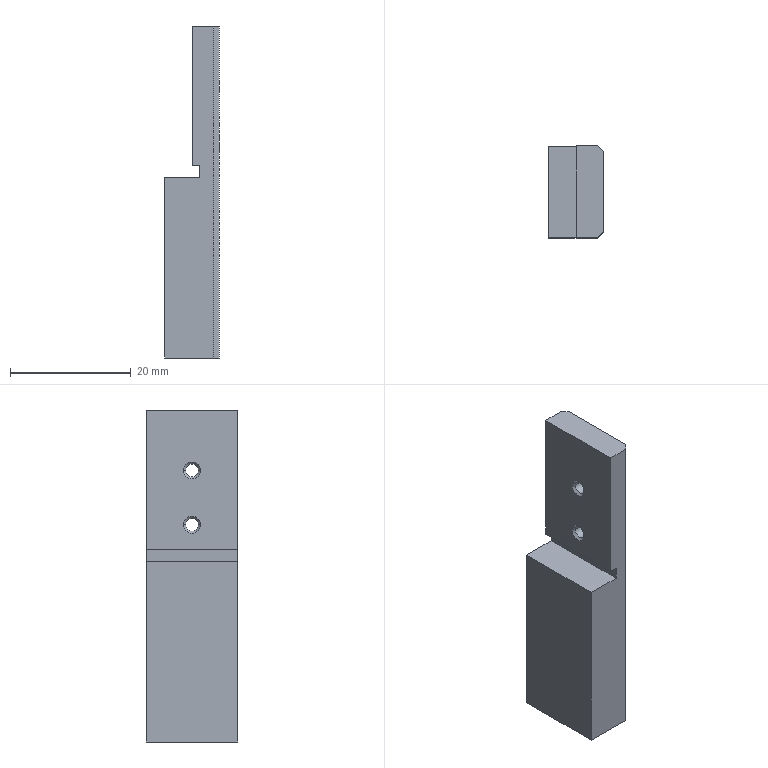Part | NX | 1 solid | 32 faces | box 9 x 15.2 x 54.9 mm | volume 5456 mm3 | plane 12 | cone 12 | cylinder 8 | commonest cylinder face diameters 2.1 x4 3.3 x4
STEP:
#1=CARTESIAN_POINT('',(7.15,0.,-23.87));
#2=VERTEX_POINT('',#1);
#3=CARTESIAN_POINT('',(1.35,0.,-23.87));
#4=VERTEX_POINT('',#3);
#5=CARTESIAN_POINT('',(0.,0.,-23.87));
#6=DIRECTION('',(-1.,0.,0.));
#7=VECTOR('',#6,1000.);
#8=LINE('',#5,#7);
#9=EDGE_CURVE('',#2,#4,#8,.T.);
#10=ORIENTED_EDGE('',*,*,#9,.T.);
#11=CARTESIAN_POINT('',(1.35,0.,-53.77));
#12=VERTEX_POINT('',#11);
#13=CARTESIAN_POINT('',(1.35,0.,0.));
#14=DIRECTION('',(0.,0.,1.));
#15=VECTOR('',#14,1000.);
#16=LINE('',#13,#15);
#17=EDGE_CURVE('',#12,#4,#16,.T.);
#18=ORIENTED_EDGE('',*,*,#17,.F.);
#19=CARTESIAN_POINT('',(9.35,0.,-53.77));
#20=VERTEX_POINT('',#19);
#21=CARTESIAN_POINT('',(0.,0.,-53.77));
#22=DIRECTION('',(-1.,0.,0.));
#23=VECTOR('',#22,1000.);
#24=LINE('',#21,#23);
#25=EDGE_CURVE('',#20,#12,#24,.T.);
#26=ORIENTED_EDGE('',*,*,#25,.F.);
#27=CARTESIAN_POINT('',(9.35,0.,1.13));
#28=VERTEX_POINT('',#27);
#29=CARTESIAN_POINT('',(9.35,0.,0.));
#30=DIRECTION('',(0.,0.,-1.));
#31=VECTOR('',#30,1000.);
#32=LINE('',#29,#31);
#33=EDGE_CURVE('',#28,#20,#32,.T.);
#34=ORIENTED_EDGE('',*,*,#33,.F.);
#35=CARTESIAN_POINT('',(5.85,0.,1.13));
#36=VERTEX_POINT('',#35);
#37=CARTESIAN_POINT('',(0.,0.,1.13));
#38=DIRECTION('',(1.,0.,0.));
#39=VECTOR('',#38,1000.);
#40=LINE('',#37,#39);
#41=EDGE_CURVE('',#36,#28,#40,.T.);
#42=ORIENTED_EDGE('',*,*,#41,.F.);
#43=CARTESIAN_POINT('',(5.85,0.,-21.87));
#44=VERTEX_POINT('',#43);
#45=CARTESIAN_POINT('',(5.85,0.,0.));
#46=DIRECTION('',(0.,0.,-1.));
#47=VECTOR('',#46,1000.);
#48=LINE('',#45,#47);
#49=EDGE_CURVE('',#36,#44,#48,.T.);
#50=ORIENTED_EDGE('',*,*,#49,.T.);
#51=CARTESIAN_POINT('',(7.15,0.,-21.87));
#52=VERTEX_POINT('',#51);
#53=CARTESIAN_POINT('',(0.,0.,-21.87));
#54=DIRECTION('',(1.,0.,0.));
#55=VECTOR('',#54,1000.);
#56=LINE('',#53,#55);
#57=EDGE_CURVE('',#44,#52,#56,.T.);
#58=ORIENTED_EDGE('',*,*,#57,.T.);
#59=CARTESIAN_POINT('',(7.15,0.,0.));
#60=DIRECTION('',(0.,0.,1.));
#61=VECTOR('',#60,1000.);
#62=LINE('',#59,#61);
#63=EDGE_CURVE('',#2,#52,#62,.T.);
#64=ORIENTED_EDGE('',*,*,#63,.F.);
#65=EDGE_LOOP('',(#10,#18,#26,#34,#42,#50,#58,#64));
#66=FACE_BOUND('',#65,.T.);
#67=CARTESIAN_POINT('',(0.,0.,0.));
#68=DIRECTION('',(0.,-1.,0.));
#69=DIRECTION('',(0.,0.,-1.));
#70=AXIS2_PLACEMENT_3D('',#67,#68,#69);
#71=PLANE('',#70);
#72=ADVANCED_FACE('',(#66),#71,.T.);
#73=ORIENTED_EDGE('',*,*,#9,.F.);
#74=CARTESIAN_POINT('',(7.15,15.2,-23.87));
#75=VERTEX_POINT('',#74);
#76=CARTESIAN_POINT('',(7.15,0.,-23.87));
#77=DIRECTION('',(0.,-1.,0.));
#78=VECTOR('',#77,1000.);
#79=LINE('',#76,#78);
#80=EDGE_CURVE('',#75,#2,#79,.T.);
#81=ORIENTED_EDGE('',*,*,#80,.F.);
#82=CARTESIAN_POINT('',(1.35,15.2,-23.87));
#83=VERTEX_POINT('',#82);
#84=CARTESIAN_POINT('',(0.,15.2,-23.87));
#85=DIRECTION('',(1.,0.,0.));
#86=VECTOR('',#85,1000.);
#87=LINE('',#84,#86);
#88=EDGE_CURVE('',#83,#75,#87,.T.);
#89=ORIENTED_EDGE('',*,*,#88,.F.);
#90=CARTESIAN_POINT('',(1.35,0.,-23.87));
#91=DIRECTION('',(0.,-1.,0.));
#92=VECTOR('',#91,1000.);
#93=LINE('',#90,#92);
#94=EDGE_CURVE('',#83,#4,#93,.T.);
#95=ORIENTED_EDGE('',*,*,#94,.T.);
#96=EDGE_LOOP('',(#73,#81,#89,#95));
#97=FACE_BOUND('',#96,.T.);
#98=CARTESIAN_POINT('',(6.05,15.2,-23.87));
#99=DIRECTION('',(0.,0.,-1.));
#100=DIRECTION('',(0.,-1.,0.));
#101=AXIS2_PLACEMENT_3D('',#98,#99,#100);
#102=PLANE('',#101);
#103=ADVANCED_FACE('',(#97),#102,.F.);
#104=ORIENTED_EDGE('',*,*,#94,.F.);
#105=CARTESIAN_POINT('',(1.35,15.2,-53.77));
#106=VERTEX_POINT('',#105);
#107=CARTESIAN_POINT('',(1.35,15.2,0.));
#108=DIRECTION('',(0.,0.,-1.));
#109=VECTOR('',#108,1000.);
#110=LINE('',#107,#109);
#111=EDGE_CURVE('',#83,#106,#110,.T.);
#112=ORIENTED_EDGE('',*,*,#111,.T.);
#113=CARTESIAN_POINT('',(1.35,0.,-53.77));
#114=DIRECTION('',(0.,-1.,0.));
#115=VECTOR('',#114,1000.);
#116=LINE('',#113,#115);
#117=EDGE_CURVE('',#106,#12,#116,.T.);
#118=ORIENTED_EDGE('',*,*,#117,.T.);
#119=ORIENTED_EDGE('',*,*,#17,.T.);
#120=EDGE_LOOP('',(#104,#112,#118,#119));
#121=FACE_BOUND('',#120,.T.);
#122=CARTESIAN_POINT('',(1.35,0.,1.13));
#123=DIRECTION('',(-1.,0.,0.));
#124=DIRECTION('',(0.,0.,1.));
#125=AXIS2_PLACEMENT_3D('',#122,#123,#124);
#126=PLANE('',#125);
#127=ADVANCED_FACE('',(#121),#126,.T.);
#128=ORIENTED_EDGE('',*,*,#49,.F.);
#129=CARTESIAN_POINT('',(5.85,15.2,1.13));
#130=VERTEX_POINT('',#129);
#131=CARTESIAN_POINT('',(5.85,0.,1.13));
#132=DIRECTION('',(0.,1.,0.));
#133=VECTOR('',#132,1000.);
#134=LINE('',#131,#133);
#135=EDGE_CURVE('',#36,#130,#134,.T.);
#136=ORIENTED_EDGE('',*,*,#135,.T.);
#137=CARTESIAN_POINT('',(5.85,15.2,-21.87));
#138=VERTEX_POINT('',#137);
#139=CARTESIAN_POINT('',(5.85,15.2,0.));
#140=DIRECTION('',(0.,0.,1.));
#141=VECTOR('',#140,1000.);
#142=LINE('',#139,#141);
#143=EDGE_CURVE('',#138,#130,#142,.T.);
#144=ORIENTED_EDGE('',*,*,#143,.F.);
#145=CARTESIAN_POINT('',(5.85,0.,-21.87));
#146=DIRECTION('',(0.,-1.,0.));
#147=VECTOR('',#146,1000.);
#148=LINE('',#145,#147);
#149=EDGE_CURVE('',#138,#44,#148,.T.);
#150=ORIENTED_EDGE('',*,*,#149,.T.);
#151=EDGE_LOOP('',(#128,#136,#144,#150));
#152=FACE_BOUND('',#151,.T.);
#153=CARTESIAN_POINT('',(5.85,9.,-17.87));
#154=VERTEX_POINT('',#153);
#155=CARTESIAN_POINT('',(5.85,6.2,-17.87));
#156=VERTEX_POINT('',#155);
#157=CARTESIAN_POINT('',(5.85,7.6,-17.87));
#158=DIRECTION('',(-1.,0.,0.));
#159=DIRECTION('',(0.,1.,0.));
#160=AXIS2_PLACEMENT_3D('',#157,#158,#159);
#161=CIRCLE('',#160,1.4);
#162=EDGE_CURVE('',#154,#156,#161,.T.);
#163=ORIENTED_EDGE('',*,*,#162,.F.);
#164=CARTESIAN_POINT('',(5.85,7.6,-17.87));
#165=DIRECTION('',(-1.,0.,0.));
#166=DIRECTION('',(0.,1.,0.));
#167=AXIS2_PLACEMENT_3D('',#164,#165,#166);
#168=CIRCLE('',#167,1.4);
#169=EDGE_CURVE('',#156,#154,#168,.T.);
#170=ORIENTED_EDGE('',*,*,#169,.F.);
#171=EDGE_LOOP('',(#163,#170));
#172=FACE_BOUND('',#171,.T.);
#173=CARTESIAN_POINT('',(5.85,9.,-8.87));
#174=VERTEX_POINT('',#173);
#175=CARTESIAN_POINT('',(5.85,6.2,-8.87));
#176=VERTEX_POINT('',#175);
#177=CARTESIAN_POINT('',(5.85,7.6,-8.87));
#178=DIRECTION('',(-1.,0.,0.));
#179=DIRECTION('',(0.,1.,0.));
#180=AXIS2_PLACEMENT_3D('',#177,#178,#179);
#181=CIRCLE('',#180,1.4);
#182=EDGE_CURVE('',#174,#176,#181,.T.);
#183=ORIENTED_EDGE('',*,*,#182,.F.);
#184=CARTESIAN_POINT('',(5.85,7.6,-8.87));
#185=DIRECTION('',(-1.,0.,0.));
#186=DIRECTION('',(0.,1.,0.));
#187=AXIS2_PLACEMENT_3D('',#184,#185,#186);
#188=CIRCLE('',#187,1.4);
#189=EDGE_CURVE('',#176,#174,#188,.T.);
#190=ORIENTED_EDGE('',*,*,#189,.F.);
#191=EDGE_LOOP('',(#183,#190));
#192=FACE_BOUND('',#191,.T.);
#193=CARTESIAN_POINT('',(5.85,15.2,1.13));
#194=DIRECTION('',(1.,0.,0.));
#195=DIRECTION('',(0.,1.,0.));
#196=AXIS2_PLACEMENT_3D('',#193,#194,#195);
#197=PLANE('',#196);
#198=ADVANCED_FACE('',(#152,#172,#192),#197,.F.);
#199=ORIENTED_EDGE('',*,*,#88,.T.);
#200=CARTESIAN_POINT('',(7.15,15.2,-21.87));
#201=VERTEX_POINT('',#200);
#202=CARTESIAN_POINT('',(7.15,15.2,0.));
#203=DIRECTION('',(0.,0.,1.));
#204=VECTOR('',#203,1000.);
#205=LINE('',#202,#204);
#206=EDGE_CURVE('',#75,#201,#205,.T.);
#207=ORIENTED_EDGE('',*,*,#206,.T.);
#208=CARTESIAN_POINT('',(0.,15.2,-21.87));
#209=DIRECTION('',(-1.,0.,0.));
#210=VECTOR('',#209,1000.);
#211=LINE('',#208,#210);
#212=EDGE_CURVE('',#201,#138,#211,.T.);
#213=ORIENTED_EDGE('',*,*,#212,.T.);
#214=ORIENTED_EDGE('',*,*,#143,.T.);
#215=CARTESIAN_POINT('',(9.35,15.2,1.13));
#216=VERTEX_POINT('',#215);
#217=CARTESIAN_POINT('',(0.,15.2,1.13));
#218=DIRECTION('',(-1.,0.,0.));
#219=VECTOR('',#218,1000.);
#220=LINE('',#217,#219);
#221=EDGE_CURVE('',#216,#130,#220,.T.);
#222=ORIENTED_EDGE('',*,*,#221,.F.);
#223=CARTESIAN_POINT('',(9.35,15.2,-53.77));
#224=VERTEX_POINT('',#223);
#225=CARTESIAN_POINT('',(9.35,15.2,0.));
#226=DIRECTION('',(0.,0.,1.));
#227=VECTOR('',#226,1000.);
#228=LINE('',#225,#227);
#229=EDGE_CURVE('',#224,#216,#228,.T.);
#230=ORIENTED_EDGE('',*,*,#229,.F.);
#231=CARTESIAN_POINT('',(0.,15.2,-53.77));
#232=DIRECTION('',(1.,0.,0.));
#233=VECTOR('',#232,1000.);
#234=LINE('',#231,#233);
#235=EDGE_CURVE('',#106,#224,#234,.T.);
#236=ORIENTED_EDGE('',*,*,#235,.F.);
#237=ORIENTED_EDGE('',*,*,#111,.F.);
#238=EDGE_LOOP('',(#199,#207,#213,#214,#222,#230,#236,#237));
#239=FACE_BOUND('',#238,.T.);
#240=CARTESIAN_POINT('',(1.35,15.2,0.));
#241=DIRECTION('',(0.,1.,0.));
#242=DIRECTION('',(1.,0.,0.));
#243=AXIS2_PLACEMENT_3D('',#240,#241,#242);
#244=PLANE('',#243);
#245=ADVANCED_FACE('',(#239),#244,.T.);
#246=CARTESIAN_POINT('',(10.35,14.2,-53.77));
#247=VERTEX_POINT('',#246);
#248=CARTESIAN_POINT('',(10.35,14.2,1.13));
#249=VERTEX_POINT('',#248);
#250=CARTESIAN_POINT('',(10.35,14.2,-53.77));
#251=DIRECTION('',(0.,0.,1.));
#252=VECTOR('',#251,1000.);
#253=LINE('',#250,#252);
#254=EDGE_CURVE('',#247,#249,#253,.T.);
#255=ORIENTED_EDGE('',*,*,#254,.F.);
#256=CARTESIAN_POINT('',(24.55,0.,-53.77));
#257=DIRECTION('',(-0.7071,0.7071,0.));
#258=VECTOR('',#257,1000.);
#259=LINE('',#256,#258);
#260=EDGE_CURVE('',#247,#224,#259,.T.);
#261=ORIENTED_EDGE('',*,*,#260,.T.);
#262=ORIENTED_EDGE('',*,*,#229,.T.);
#263=CARTESIAN_POINT('',(24.55,0.,1.13));
#264=DIRECTION('',(0.7071,-0.7071,0.));
#265=VECTOR('',#264,1000.);
#266=LINE('',#263,#265);
#267=EDGE_CURVE('',#216,#249,#266,.T.);
#268=ORIENTED_EDGE('',*,*,#267,.T.);
#269=EDGE_LOOP('',(#255,#261,#262,#268));
#270=FACE_BOUND('',#269,.T.);
#271=CARTESIAN_POINT('',(10.35,14.2,1.13));
#272=DIRECTION('',(0.7071,0.7071,0.));
#273=DIRECTION('',(0.,0.,-1.));
#274=AXIS2_PLACEMENT_3D('',#271,#272,#273);
#275=PLANE('',#274);
#276=ADVANCED_FACE('',(#270),#275,.T.);
#277=CARTESIAN_POINT('',(10.35,1.,1.13));
#278=VERTEX_POINT('',#277);
#279=CARTESIAN_POINT('',(10.35,0.,1.13));
#280=DIRECTION('',(0.,-1.,0.));
#281=VECTOR('',#280,1000.);
#282=LINE('',#279,#281);
#283=EDGE_CURVE('',#249,#278,#282,.T.);
#284=ORIENTED_EDGE('',*,*,#283,.T.);
#285=CARTESIAN_POINT('',(10.35,1.,-53.77));
#286=VERTEX_POINT('',#285);
#287=CARTESIAN_POINT('',(10.35,1.,-53.77));
#288=DIRECTION('',(0.,0.,1.));
#289=VECTOR('',#288,1000.);
#290=LINE('',#287,#289);
#291=EDGE_CURVE('',#286,#278,#290,.T.);
#292=ORIENTED_EDGE('',*,*,#291,.F.);
#293=CARTESIAN_POINT('',(10.35,0.,-53.77));
#294=DIRECTION('',(0.,1.,0.));
#295=VECTOR('',#294,1000.);
#296=LINE('',#293,#295);
#297=EDGE_CURVE('',#286,#247,#296,.T.);
#298=ORIENTED_EDGE('',*,*,#297,.T.);
#299=ORIENTED_EDGE('',*,*,#254,.T.);
#300=EDGE_LOOP('',(#284,#292,#298,#299));
#301=FACE_BOUND('',#300,.T.);
#302=CARTESIAN_POINT('',(10.35,8.65,-17.87));
#303=VERTEX_POINT('',#302);
#304=CARTESIAN_POINT('',(10.35,6.55,-17.87));
#305=VERTEX_POINT('',#304);
#306=CARTESIAN_POINT('',(10.35,7.6,-17.87));
#307=DIRECTION('',(-1.,0.,0.));
#308=DIRECTION('',(0.,1.,0.));
#309=AXIS2_PLACEMENT_3D('',#306,#307,#308);
#310=CIRCLE('',#309,1.05);
#311=EDGE_CURVE('',#303,#305,#310,.T.);
#312=ORIENTED_EDGE('',*,*,#311,.T.);
#313=CARTESIAN_POINT('',(10.35,7.6,-17.87));
#314=DIRECTION('',(-1.,0.,0.));
#315=DIRECTION('',(0.,1.,0.));
#316=AXIS2_PLACEMENT_3D('',#313,#314,#315);
#317=CIRCLE('',#316,1.05);
#318=EDGE_CURVE('',#305,#303,#317,.T.);
#319=ORIENTED_EDGE('',*,*,#318,.T.);
#320=EDGE_LOOP('',(#312,#319));
#321=FACE_BOUND('',#320,.T.);
#322=CARTESIAN_POINT('',(10.35,8.65,-8.87));
#323=VERTEX_POINT('',#322);
#324=CARTESIAN_POINT('',(10.35,6.55,-8.87));
#325=VERTEX_POINT('',#324);
#326=CARTESIAN_POINT('',(10.35,7.6,-8.87));
#327=DIRECTION('',(-1.,0.,0.));
#328=DIRECTION('',(0.,1.,0.));
#329=AXIS2_PLACEMENT_3D('',#326,#327,#328);
#330=CIRCLE('',#329,1.05);
#331=EDGE_CURVE('',#323,#325,#330,.T.);
#332=ORIENTED_EDGE('',*,*,#331,.T.);
#333=CARTESIAN_POINT('',(10.35,7.6,-8.87));
#334=DIRECTION('',(-1.,0.,0.));
#335=DIRECTION('',(0.,1.,0.));
#336=AXIS2_PLACEMENT_3D('',#333,#334,#335);
#337=CIRCLE('',#336,1.05);
#338=EDGE_CURVE('',#325,#323,#337,.T.);
#339=ORIENTED_EDGE('',*,*,#338,.T.);
#340=EDGE_LOOP('',(#332,#339));
#341=FACE_BOUND('',#340,.T.);
#342=CARTESIAN_POINT('',(10.35,15.2,1.13));
#343=DIRECTION('',(1.,0.,0.));
#344=DIRECTION('',(0.,1.,0.));
#345=AXIS2_PLACEMENT_3D('',#342,#343,#344);
#346=PLANE('',#345);
#347=ADVANCED_FACE('',(#301,#321,#341),#346,.T.);
#348=ORIENTED_EDGE('',*,*,#135,.F.);
#349=ORIENTED_EDGE('',*,*,#41,.T.);
#350=CARTESIAN_POINT('',(9.35,0.,1.13));
#351=DIRECTION('',(-0.7071,-0.7071,0.));
#352=VECTOR('',#351,1000.);
#353=LINE('',#350,#352);
#354=EDGE_CURVE('',#278,#28,#353,.T.);
#355=ORIENTED_EDGE('',*,*,#354,.F.);
#356=ORIENTED_EDGE('',*,*,#283,.F.);
#357=ORIENTED_EDGE('',*,*,#267,.F.);
#358=ORIENTED_EDGE('',*,*,#221,.T.);
#359=EDGE_LOOP('',(#348,#349,#355,#356,#357,#358));
#360=FACE_BOUND('',#359,.T.);
#361=CARTESIAN_POINT('',(0.,0.,1.13));
#362=DIRECTION('',(0.,0.,1.));
#363=DIRECTION('',(1.,0.,0.));
#364=AXIS2_PLACEMENT_3D('',#361,#362,#363);
#365=PLANE('',#364);
#366=ADVANCED_FACE('',(#360),#365,.T.);
#367=ORIENTED_EDGE('',*,*,#235,.T.);
#368=ORIENTED_EDGE('',*,*,#260,.F.);
#369=ORIENTED_EDGE('',*,*,#297,.F.);
#370=CARTESIAN_POINT('',(9.35,0.,-53.77));
#371=DIRECTION('',(0.7071,0.7071,0.));
#372=VECTOR('',#371,1000.);
#373=LINE('',#370,#372);
#374=EDGE_CURVE('',#20,#286,#373,.T.);
#375=ORIENTED_EDGE('',*,*,#374,.F.);
#376=ORIENTED_EDGE('',*,*,#25,.T.);
#377=ORIENTED_EDGE('',*,*,#117,.F.);
#378=EDGE_LOOP('',(#367,#368,#369,#375,#376,#377));
#379=FACE_BOUND('',#378,.T.);
#380=CARTESIAN_POINT('',(8.165,3.,-53.77));
#381=VERTEX_POINT('',#380);
#382=CARTESIAN_POINT('',(3.535,3.,-53.77));
#383=VERTEX_POINT('',#382);
#384=CARTESIAN_POINT('',(5.85,3.,-53.77));
#385=DIRECTION('',(0.,0.,-1.));
#386=DIRECTION('',(-1.,0.,0.));
#387=AXIS2_PLACEMENT_3D('',#384,#385,#386);
#388=CIRCLE('',#387,2.315);
#389=EDGE_CURVE('',#381,#383,#388,.T.);
#390=ORIENTED_EDGE('',*,*,#389,.F.);
#391=CARTESIAN_POINT('',(5.85,3.,-53.77));
#392=DIRECTION('',(0.,0.,-1.));
#393=DIRECTION('',(-1.,0.,0.));
#394=AXIS2_PLACEMENT_3D('',#391,#392,#393);
#395=CIRCLE('',#394,2.315);
#396=EDGE_CURVE('',#383,#381,#395,.T.);
#397=ORIENTED_EDGE('',*,*,#396,.F.);
#398=EDGE_LOOP('',(#390,#397));
#399=FACE_BOUND('',#398,.T.);
#400=CARTESIAN_POINT('',(8.165,12.2,-53.77));
#401=VERTEX_POINT('',#400);
#402=CARTESIAN_POINT('',(3.535,12.2,-53.77));
#403=VERTEX_POINT('',#402);
#404=CARTESIAN_POINT('',(5.85,12.2,-53.77));
#405=DIRECTION('',(0.,0.,-1.));
#406=DIRECTION('',(-1.,0.,0.));
#407=AXIS2_PLACEMENT_3D('',#404,#405,#406);
#408=CIRCLE('',#407,2.315);
#409=EDGE_CURVE('',#401,#403,#408,.T.);
#410=ORIENTED_EDGE('',*,*,#409,.F.);
#411=CARTESIAN_POINT('',(5.85,12.2,-53.77));
#412=DIRECTION('',(0.,0.,-1.));
#413=DIRECTION('',(-1.,0.,0.));
#414=AXIS2_PLACEMENT_3D('',#411,#412,#413);
#415=CIRCLE('',#414,2.315);
#416=EDGE_CURVE('',#403,#401,#415,.T.);
#417=ORIENTED_EDGE('',*,*,#416,.F.);
#418=EDGE_LOOP('',(#410,#417));
#419=FACE_BOUND('',#418,.T.);
#420=CARTESIAN_POINT('',(0.,0.,-53.77));
#421=DIRECTION('',(0.,0.,-1.));
#422=DIRECTION('',(0.,-1.,0.));
#423=AXIS2_PLACEMENT_3D('',#420,#421,#422);
#424=PLANE('',#423);
#425=ADVANCED_FACE('',(#379,#399,#419),#424,.T.);
#426=ORIENTED_EDGE('',*,*,#57,.F.);
#427=ORIENTED_EDGE('',*,*,#149,.F.);
#428=ORIENTED_EDGE('',*,*,#212,.F.);
#429=CARTESIAN_POINT('',(7.15,0.,-21.87));
#430=DIRECTION('',(0.,1.,0.));
#431=VECTOR('',#430,1000.);
#432=LINE('',#429,#431);
#433=EDGE_CURVE('',#52,#201,#432,.T.);
#434=ORIENTED_EDGE('',*,*,#433,.F.);
#435=EDGE_LOOP('',(#426,#427,#428,#434));
#436=FACE_BOUND('',#435,.T.);
#437=CARTESIAN_POINT('',(4.85,15.2,-21.87));
#438=DIRECTION('',(0.,0.,1.));
#439=DIRECTION('',(1.,0.,0.));
#440=AXIS2_PLACEMENT_3D('',#437,#438,#439);
#441=PLANE('',#440);
#442=ADVANCED_FACE('',(#436),#441,.F.);
#443=ORIENTED_EDGE('',*,*,#63,.T.);
#444=ORIENTED_EDGE('',*,*,#433,.T.);
#445=ORIENTED_EDGE('',*,*,#206,.F.);
#446=ORIENTED_EDGE('',*,*,#80,.T.);
#447=EDGE_LOOP('',(#443,#444,#445,#446));
#448=FACE_BOUND('',#447,.T.);
#449=CARTESIAN_POINT('',(7.15,15.2,-21.87));
#450=DIRECTION('',(1.,0.,0.));
#451=DIRECTION('',(0.,1.,0.));
#452=AXIS2_PLACEMENT_3D('',#449,#450,#451);
#453=PLANE('',#452);
#454=ADVANCED_FACE('',(#448),#453,.F.);
#455=ORIENTED_EDGE('',*,*,#311,.F.);
#456=CARTESIAN_POINT('',(6.2,8.65,-17.87));
#457=VERTEX_POINT('',#456);
#458=CARTESIAN_POINT('',(10.762,8.65,-17.87));
#459=DIRECTION('',(-1.,0.,0.));
#460=VECTOR('',#459,1000.);
#461=LINE('',#458,#460);
#462=EDGE_CURVE('',#303,#457,#461,.T.);
#463=ORIENTED_EDGE('',*,*,#462,.T.);
#464=CARTESIAN_POINT('',(6.2,6.55,-17.87));
#465=VERTEX_POINT('',#464);
#466=CARTESIAN_POINT('',(6.2,7.6,-17.87));
#467=DIRECTION('',(-1.,0.,0.));
#468=DIRECTION('',(0.,1.,0.));
#469=AXIS2_PLACEMENT_3D('',#466,#467,#468);
#470=CIRCLE('',#469,1.05);
#471=EDGE_CURVE('',#457,#465,#470,.T.);
#472=ORIENTED_EDGE('',*,*,#471,.T.);
#473=CARTESIAN_POINT('',(10.762,6.55,-17.87));
#474=DIRECTION('',(-1.,0.,0.));
#475=VECTOR('',#474,1000.);
#476=LINE('',#473,#475);
#477=EDGE_CURVE('',#305,#465,#476,.T.);
#478=ORIENTED_EDGE('',*,*,#477,.F.);
#479=EDGE_LOOP('',(#455,#463,#472,#478));
#480=FACE_BOUND('',#479,.T.);
#481=CARTESIAN_POINT('',(10.762,7.6,-17.87));
#482=DIRECTION('',(-1.,0.,0.));
#483=DIRECTION('',(0.,1.,0.));
#484=AXIS2_PLACEMENT_3D('',#481,#482,#483);
#485=CYLINDRICAL_SURFACE('',#484,1.05);
#486=ADVANCED_FACE('',(#480),#485,.F.);
#487=CARTESIAN_POINT('',(7.5,12.2,-41.57));
#488=VERTEX_POINT('',#487);
#489=CARTESIAN_POINT('',(5.85,13.85,-41.57));
#490=VERTEX_POINT('',#489);
#491=CARTESIAN_POINT('',(5.85,12.2,-41.57));
#492=DIRECTION('',(0.,0.,1.));
#493=DIRECTION('',(-1.,0.,0.));
#494=AXIS2_PLACEMENT_3D('',#491,#492,#493);
#495=CIRCLE('',#494,1.65);
#496=EDGE_CURVE('',#488,#490,#495,.T.);
#497=ORIENTED_EDGE('',*,*,#496,.T.);
#498=CARTESIAN_POINT('',(5.85,13.85,-53.386));
#499=VERTEX_POINT('',#498);
#500=CARTESIAN_POINT('',(5.85,13.85,-43.67));
#501=DIRECTION('',(0.,0.,-1.));
#502=VECTOR('',#501,1000.);
#503=LINE('',#500,#502);
#504=EDGE_CURVE('',#490,#499,#503,.T.);
#505=ORIENTED_EDGE('',*,*,#504,.T.);
#506=CARTESIAN_POINT('',(7.5,12.2,-53.386));
#507=VERTEX_POINT('',#506);
#508=CARTESIAN_POINT('',(5.85,12.2,-53.386));
#509=DIRECTION('',(0.,0.,-1.));
#510=DIRECTION('',(-1.,0.,0.));
#511=AXIS2_PLACEMENT_3D('',#508,#509,#510);
#512=CIRCLE('',#511,1.65);
#513=EDGE_CURVE('',#499,#507,#512,.T.);
#514=ORIENTED_EDGE('',*,*,#513,.T.);
#515=CARTESIAN_POINT('',(5.85,10.55,-53.386));
#516=VERTEX_POINT('',#515);
#517=CARTESIAN_POINT('',(5.85,12.2,-53.386));
#518=DIRECTION('',(0.,0.,-1.));
#519=DIRECTION('',(-1.,0.,0.));
#520=AXIS2_PLACEMENT_3D('',#517,#518,#519);
#521=CIRCLE('',#520,1.65);
#522=EDGE_CURVE('',#507,#516,#521,.T.);
#523=ORIENTED_EDGE('',*,*,#522,.T.);
#524=CARTESIAN_POINT('',(5.85,10.55,-41.57));
#525=VERTEX_POINT('',#524);
#526=CARTESIAN_POINT('',(5.85,10.55,-43.67));
#527=DIRECTION('',(0.,0.,-1.));
#528=VECTOR('',#527,1000.);
#529=LINE('',#526,#528);
#530=EDGE_CURVE('',#525,#516,#529,.T.);
#531=ORIENTED_EDGE('',*,*,#530,.F.);
#532=CARTESIAN_POINT('',(5.85,12.2,-41.57));
#533=DIRECTION('',(0.,0.,1.));
#534=DIRECTION('',(-1.,0.,0.));
#535=AXIS2_PLACEMENT_3D('',#532,#533,#534);
#536=CIRCLE('',#535,1.65);
#537=EDGE_CURVE('',#525,#488,#536,.T.);
#538=ORIENTED_EDGE('',*,*,#537,.T.);
#539=EDGE_LOOP('',(#497,#505,#514,#523,#531,#538));
#540=FACE_BOUND('',#539,.T.);
#541=CARTESIAN_POINT('',(5.85,12.2,-43.67));
#542=DIRECTION('',(0.,0.,-1.));
#543=DIRECTION('',(0.,-1.,0.));
#544=AXIS2_PLACEMENT_3D('',#541,#542,#543);
#545=CYLINDRICAL_SURFACE('',#544,1.65);
#546=ADVANCED_FACE('',(#540),#545,.F.);
#547=ORIENTED_EDGE('',*,*,#496,.F.);
#548=CARTESIAN_POINT('',(5.85,12.2,-40.579));
#549=VERTEX_POINT('',#548);
#550=CARTESIAN_POINT('',(7.5,12.2,-41.57));
#551=DIRECTION('',(0.8572,0.,-0.515));
#552=VECTOR('',#551,1000.);
#553=LINE('',#550,#552);
#554=EDGE_CURVE('',#549,#488,#553,.T.);
#555=ORIENTED_EDGE('',*,*,#554,.F.);
#556=CARTESIAN_POINT('',(4.2,12.2,-41.57));
#557=VERTEX_POINT('',#556);
#558=CARTESIAN_POINT('',(4.2,12.2,-41.57));
#559=DIRECTION('',(-0.8572,0.,-0.515));
#560=VECTOR('',#559,1000.);
#561=LINE('',#558,#560);
#562=EDGE_CURVE('',#549,#557,#561,.T.);
#563=ORIENTED_EDGE('',*,*,#562,.T.);
#564=CARTESIAN_POINT('',(5.85,12.2,-41.57));
#565=DIRECTION('',(0.,0.,1.));
#566=DIRECTION('',(-1.,0.,0.));
#567=AXIS2_PLACEMENT_3D('',#564,#565,#566);
#568=CIRCLE('',#567,1.65);
#569=EDGE_CURVE('',#490,#557,#568,.T.);
#570=ORIENTED_EDGE('',*,*,#569,.F.);
#571=EDGE_LOOP('',(#547,#555,#563,#570));
#572=FACE_BOUND('',#571,.T.);
#573=CARTESIAN_POINT('',(5.85,12.2,-41.57));
#574=DIRECTION('',(0.,0.,-1.));
#575=DIRECTION('',(-1.,0.,0.));
#576=AXIS2_PLACEMENT_3D('',#573,#574,#575);
#577=CONICAL_SURFACE('',#576,1.65,1.03);
#578=ADVANCED_FACE('',(#572),#577,.F.);
#579=ORIENTED_EDGE('',*,*,#33,.T.);
#580=ORIENTED_EDGE('',*,*,#374,.T.);
#581=ORIENTED_EDGE('',*,*,#291,.T.);
#582=ORIENTED_EDGE('',*,*,#354,.T.);
#583=EDGE_LOOP('',(#579,#580,#581,#582));
#584=FACE_BOUND('',#583,.T.);
#585=CARTESIAN_POINT('',(9.35,0.,1.13));
#586=DIRECTION('',(0.7071,-0.7071,0.));
#587=DIRECTION('',(0.,0.,-1.));
#588=AXIS2_PLACEMENT_3D('',#585,#586,#587);
#589=PLANE('',#588);
#590=ADVANCED_FACE('',(#584),#589,.T.);
#591=CARTESIAN_POINT('',(6.2,6.55,-8.87));
#592=VERTEX_POINT('',#591);
#593=CARTESIAN_POINT('',(6.2,8.65,-8.87));
#594=VERTEX_POINT('',#593);
#595=CARTESIAN_POINT('',(6.2,7.6,-8.87));
#596=DIRECTION('',(-1.,0.,0.));
#597=DIRECTION('',(0.,1.,0.));
#598=AXIS2_PLACEMENT_3D('',#595,#596,#597);
#599=CIRCLE('',#598,1.05);
#600=EDGE_CURVE('',#592,#594,#599,.T.);
#601=ORIENTED_EDGE('',*,*,#600,.T.);
#602=CARTESIAN_POINT('',(11.25,8.65,-8.87));
#603=DIRECTION('',(-1.,0.,0.));
#604=VECTOR('',#603,1000.);
#605=LINE('',#602,#604);
#606=EDGE_CURVE('',#323,#594,#605,.T.);
#607=ORIENTED_EDGE('',*,*,#606,.F.);
#608=ORIENTED_EDGE('',*,*,#338,.F.);
#609=CARTESIAN_POINT('',(11.25,6.55,-8.87));
#610=DIRECTION('',(-1.,0.,0.));
#611=VECTOR('',#610,1000.);
#612=LINE('',#609,#611);
#613=EDGE_CURVE('',#325,#592,#612,.T.);
#614=ORIENTED_EDGE('',*,*,#613,.T.);
#615=EDGE_LOOP('',(#601,#607,#608,#614));
#616=FACE_BOUND('',#615,.T.);
#617=CARTESIAN_POINT('',(11.25,7.6,-8.87));
#618=DIRECTION('',(-1.,0.,0.));
#619=DIRECTION('',(0.,1.,0.));
#620=AXIS2_PLACEMENT_3D('',#617,#618,#619);
#621=CYLINDRICAL_SURFACE('',#620,1.05);
#622=ADVANCED_FACE('',(#616),#621,.F.);
#623=CARTESIAN_POINT('',(5.85,4.65,-41.57));
#624=VERTEX_POINT('',#623);
#625=CARTESIAN_POINT('',(4.2,3.,-41.57));
#626=VERTEX_POINT('',#625);
#627=CARTESIAN_POINT('',(5.85,3.,-41.57));
#628=DIRECTION('',(0.,0.,1.));
#629=DIRECTION('',(-1.,0.,0.));
#630=AXIS2_PLACEMENT_3D('',#627,#628,#629);
#631=CIRCLE('',#630,1.65);
#632=EDGE_CURVE('',#624,#626,#631,.T.);
#633=ORIENTED_EDGE('',*,*,#632,.T.);
#634=CARTESIAN_POINT('',(5.85,1.35,-41.57));
#635=VERTEX_POINT('',#634);
#636=CARTESIAN_POINT('',(5.85,3.,-41.57));
#637=DIRECTION('',(0.,0.,1.));
#638=DIRECTION('',(-1.,0.,0.));
#639=AXIS2_PLACEMENT_3D('',#636,#637,#638);
#640=CIRCLE('',#639,1.65);
#641=EDGE_CURVE('',#626,#635,#640,.T.);
#642=ORIENTED_EDGE('',*,*,#641,.T.);
#643=CARTESIAN_POINT('',(5.85,1.35,-53.386));
#644=VERTEX_POINT('',#643);
#645=CARTESIAN_POINT('',(5.85,1.35,-49.77));
#646=DIRECTION('',(0.,0.,-1.));
#647=VECTOR('',#646,1000.);
#648=LINE('',#645,#647);
#649=EDGE_CURVE('',#644,#635,#648,.F.);
#650=ORIENTED_EDGE('',*,*,#649,.F.);
#651=CARTESIAN_POINT('',(4.2,3.,-53.386));
#652=VERTEX_POINT('',#651);
#653=CARTESIAN_POINT('',(5.85,3.,-53.386));
#654=DIRECTION('',(0.,0.,-1.));
#655=DIRECTION('',(-1.,0.,0.));
#656=AXIS2_PLACEMENT_3D('',#653,#654,#655);
#657=CIRCLE('',#656,1.65);
#658=EDGE_CURVE('',#644,#652,#657,.T.);
#659=ORIENTED_EDGE('',*,*,#658,.T.);
#660=CARTESIAN_POINT('',(5.85,4.65,-53.386));
#661=VERTEX_POINT('',#660);
#662=CARTESIAN_POINT('',(5.85,3.,-53.386));
#663=DIRECTION('',(0.,0.,-1.));
#664=DIRECTION('',(-1.,0.,0.));
#665=AXIS2_PLACEMENT_3D('',#662,#663,#664);
#666=CIRCLE('',#665,1.65);
#667=EDGE_CURVE('',#652,#661,#666,.T.);
#668=ORIENTED_EDGE('',*,*,#667,.T.);
#669=CARTESIAN_POINT('',(5.85,4.65,-49.77));
#670=DIRECTION('',(0.,0.,-1.));
#671=VECTOR('',#670,1000.);
#672=LINE('',#669,#671);
#673=EDGE_CURVE('',#661,#624,#672,.F.);
#674=ORIENTED_EDGE('',*,*,#673,.T.);
#675=EDGE_LOOP('',(#633,#642,#650,#659,#668,#674));
#676=FACE_BOUND('',#675,.T.);
#677=CARTESIAN_POINT('',(5.85,3.,-49.77));
#678=DIRECTION('',(0.,0.,-1.));
#679=DIRECTION('',(0.,-1.,0.));
#680=AXIS2_PLACEMENT_3D('',#677,#678,#679);
#681=CYLINDRICAL_SURFACE('',#680,1.65);
#682=ADVANCED_FACE('',(#676),#681,.F.);
#683=ORIENTED_EDGE('',*,*,#389,.T.);
#684=CARTESIAN_POINT('',(3.535,3.,-53.77));
#685=DIRECTION('',(-0.866,0.,-0.5));
#686=VECTOR('',#685,1000.);
#687=LINE('',#684,#686);
#688=EDGE_CURVE('',#383,#652,#687,.F.);
#689=ORIENTED_EDGE('',*,*,#688,.T.);
#690=ORIENTED_EDGE('',*,*,#658,.F.);
#691=CARTESIAN_POINT('',(7.5,3.,-53.386));
#692=VERTEX_POINT('',#691);
#693=CARTESIAN_POINT('',(5.85,3.,-53.386));
#694=DIRECTION('',(0.,0.,-1.));
#695=DIRECTION('',(-1.,0.,0.));
#696=AXIS2_PLACEMENT_3D('',#693,#694,#695);
#697=CIRCLE('',#696,1.65);
#698=EDGE_CURVE('',#692,#644,#697,.T.);
#699=ORIENTED_EDGE('',*,*,#698,.F.);
#700=CARTESIAN_POINT('',(8.165,3.,-53.77));
#701=DIRECTION('',(0.866,0.,-0.5));
#702=VECTOR('',#701,1000.);
#703=LINE('',#700,#702);
#704=EDGE_CURVE('',#381,#692,#703,.F.);
#705=ORIENTED_EDGE('',*,*,#704,.F.);
#706=EDGE_LOOP('',(#683,#689,#690,#699,#705));
#707=FACE_BOUND('',#706,.T.);
#708=CARTESIAN_POINT('',(5.85,3.,-53.77));
#709=DIRECTION('',(0.,0.,-1.));
#710=DIRECTION('',(-1.,0.,0.));
#711=AXIS2_PLACEMENT_3D('',#708,#709,#710);
#712=CONICAL_SURFACE('',#711,2.315,1.047);
#713=ADVANCED_FACE('',(#707),#712,.F.);
#714=ORIENTED_EDGE('',*,*,#182,.T.);
#715=CARTESIAN_POINT('',(5.85,6.2,-8.87));
#716=DIRECTION('',(-0.7071,-0.7071,0.));
#717=VECTOR('',#716,1000.);
#718=LINE('',#715,#717);
#719=EDGE_CURVE('',#176,#592,#718,.F.);
#720=ORIENTED_EDGE('',*,*,#719,.T.);
#721=CARTESIAN_POINT('',(6.2,7.6,-8.87));
#722=DIRECTION('',(-1.,0.,0.));
#723=DIRECTION('',(0.,1.,0.));
#724=AXIS2_PLACEMENT_3D('',#721,#722,#723);
#725=CIRCLE('',#724,1.05);
#726=EDGE_CURVE('',#594,#592,#725,.T.);
#727=ORIENTED_EDGE('',*,*,#726,.F.);
#728=CARTESIAN_POINT('',(5.85,9.,-8.87));
#729=DIRECTION('',(-0.7071,0.7071,0.));
#730=VECTOR('',#729,1000.);
#731=LINE('',#728,#730);
#732=EDGE_CURVE('',#174,#594,#731,.F.);
#733=ORIENTED_EDGE('',*,*,#732,.F.);
#734=EDGE_LOOP('',(#714,#720,#727,#733));
#735=FACE_BOUND('',#734,.T.);
#736=CARTESIAN_POINT('',(5.85,7.6,-8.87));
#737=DIRECTION('',(-1.,0.,0.));
#738=DIRECTION('',(0.,1.,0.));
#739=AXIS2_PLACEMENT_3D('',#736,#737,#738);
#740=CONICAL_SURFACE('',#739,1.4,0.7854);
#741=ADVANCED_FACE('',(#735),#740,.F.);
#742=CARTESIAN_POINT('',(5.85,3.,-40.579));
#743=VERTEX_POINT('',#742);
#744=CARTESIAN_POINT('',(7.5,3.,-41.57));
#745=VERTEX_POINT('',#744);
#746=CARTESIAN_POINT('',(7.5,3.,-41.57));
#747=DIRECTION('',(0.8572,0.,-0.515));
#748=VECTOR('',#747,1000.);
#749=LINE('',#746,#748);
#750=EDGE_CURVE('',#743,#745,#749,.T.);
#751=ORIENTED_EDGE('',*,*,#750,.T.);
#752=CARTESIAN_POINT('',(5.85,3.,-41.57));
#753=DIRECTION('',(0.,0.,1.));
#754=DIRECTION('',(-1.,0.,0.));
#755=AXIS2_PLACEMENT_3D('',#752,#753,#754);
#756=CIRCLE('',#755,1.65);
#757=EDGE_CURVE('',#635,#745,#756,.T.);
#758=ORIENTED_EDGE('',*,*,#757,.F.);
#759=ORIENTED_EDGE('',*,*,#641,.F.);
#760=CARTESIAN_POINT('',(4.2,3.,-41.57));
#761=DIRECTION('',(-0.8572,0.,-0.515));
#762=VECTOR('',#761,1000.);
#763=LINE('',#760,#762);
#764=EDGE_CURVE('',#743,#626,#763,.T.);
#765=ORIENTED_EDGE('',*,*,#764,.F.);
#766=EDGE_LOOP('',(#751,#758,#759,#765));
#767=FACE_BOUND('',#766,.T.);
#768=CARTESIAN_POINT('',(5.85,3.,-41.57));
#769=DIRECTION('',(0.,0.,-1.));
#770=DIRECTION('',(-1.,0.,0.));
#771=AXIS2_PLACEMENT_3D('',#768,#769,#770);
#772=CONICAL_SURFACE('',#771,1.65,1.03);
#773=ADVANCED_FACE('',(#767),#772,.F.);
#774=CARTESIAN_POINT('',(6.2,7.6,-17.87));
#775=DIRECTION('',(-1.,0.,0.));
#776=DIRECTION('',(0.,1.,0.));
#777=AXIS2_PLACEMENT_3D('',#774,#775,#776);
#778=CIRCLE('',#777,1.05);
#779=EDGE_CURVE('',#465,#457,#778,.T.);
#780=ORIENTED_EDGE('',*,*,#779,.F.);
#781=CARTESIAN_POINT('',(5.85,6.2,-17.87));
#782=DIRECTION('',(-0.7071,-0.7071,0.));
#783=VECTOR('',#782,1000.);
#784=LINE('',#781,#783);
#785=EDGE_CURVE('',#156,#465,#784,.F.);
#786=ORIENTED_EDGE('',*,*,#785,.F.);
#787=ORIENTED_EDGE('',*,*,#169,.T.);
#788=CARTESIAN_POINT('',(5.85,9.,-17.87));
#789=DIRECTION('',(-0.7071,0.7071,0.));
#790=VECTOR('',#789,1000.);
#791=LINE('',#788,#790);
#792=EDGE_CURVE('',#154,#457,#791,.F.);
#793=ORIENTED_EDGE('',*,*,#792,.T.);
#794=EDGE_LOOP('',(#780,#786,#787,#793));
#795=FACE_BOUND('',#794,.T.);
#796=CARTESIAN_POINT('',(5.85,7.6,-17.87));
#797=DIRECTION('',(-1.,0.,0.));
#798=DIRECTION('',(0.,1.,0.));
#799=AXIS2_PLACEMENT_3D('',#796,#797,#798);
#800=CONICAL_SURFACE('',#799,1.4,0.7854);
#801=ADVANCED_FACE('',(#795),#800,.F.);
#802=ORIENTED_EDGE('',*,*,#522,.F.);
#803=CARTESIAN_POINT('',(7.5,12.2,-53.386));
#804=DIRECTION('',(0.866,0.,-0.5));
#805=VECTOR('',#804,1000.);
#806=LINE('',#803,#805);
#807=EDGE_CURVE('',#401,#507,#806,.F.);
#808=ORIENTED_EDGE('',*,*,#807,.F.);
#809=ORIENTED_EDGE('',*,*,#409,.T.);
#810=CARTESIAN_POINT('',(4.2,12.2,-53.386));
#811=VERTEX_POINT('',#810);
#812=CARTESIAN_POINT('',(4.2,12.2,-53.386));
#813=DIRECTION('',(-0.866,0.,-0.5));
#814=VECTOR('',#813,1000.);
#815=LINE('',#812,#814);
#816=EDGE_CURVE('',#403,#811,#815,.F.);
#817=ORIENTED_EDGE('',*,*,#816,.T.);
#818=CARTESIAN_POINT('',(5.85,12.2,-53.386));
#819=DIRECTION('',(0.,0.,-1.));
#820=DIRECTION('',(-1.,0.,0.));
#821=AXIS2_PLACEMENT_3D('',#818,#819,#820);
#822=CIRCLE('',#821,1.65);
#823=EDGE_CURVE('',#516,#811,#822,.T.);
#824=ORIENTED_EDGE('',*,*,#823,.F.);
#825=EDGE_LOOP('',(#802,#808,#809,#817,#824));
#826=FACE_BOUND('',#825,.T.);
#827=CARTESIAN_POINT('',(5.85,12.2,-53.386));
#828=DIRECTION('',(0.,0.,-1.));
#829=DIRECTION('',(-1.,0.,0.));
#830=AXIS2_PLACEMENT_3D('',#827,#828,#829);
#831=CONICAL_SURFACE('',#830,1.65,1.047);
#832=ADVANCED_FACE('',(#826),#831,.F.);
#833=ORIENTED_EDGE('',*,*,#331,.F.);
#834=ORIENTED_EDGE('',*,*,#606,.T.);
#835=ORIENTED_EDGE('',*,*,#726,.T.);
#836=ORIENTED_EDGE('',*,*,#613,.F.);
#837=EDGE_LOOP('',(#833,#834,#835,#836));
#838=FACE_BOUND('',#837,.T.);
#839=CARTESIAN_POINT('',(11.25,7.6,-8.87));
#840=DIRECTION('',(-1.,0.,0.));
#841=DIRECTION('',(0.,1.,0.));
#842=AXIS2_PLACEMENT_3D('',#839,#840,#841);
#843=CYLINDRICAL_SURFACE('',#842,1.05);
#844=ADVANCED_FACE('',(#838),#843,.F.);
#845=ORIENTED_EDGE('',*,*,#504,.F.);
#846=ORIENTED_EDGE('',*,*,#569,.T.);
#847=CARTESIAN_POINT('',(5.85,12.2,-41.57));
#848=DIRECTION('',(0.,0.,1.));
#849=DIRECTION('',(-1.,0.,0.));
#850=AXIS2_PLACEMENT_3D('',#847,#848,#849);
#851=CIRCLE('',#850,1.65);
#852=EDGE_CURVE('',#557,#525,#851,.T.);
#853=ORIENTED_EDGE('',*,*,#852,.T.);
#854=ORIENTED_EDGE('',*,*,#530,.T.);
#855=ORIENTED_EDGE('',*,*,#823,.T.);
#856=CARTESIAN_POINT('',(5.85,12.2,-53.386));
#857=DIRECTION('',(0.,0.,-1.));
#858=DIRECTION('',(-1.,0.,0.));
#859=AXIS2_PLACEMENT_3D('',#856,#857,#858);
#860=CIRCLE('',#859,1.65);
#861=EDGE_CURVE('',#811,#499,#860,.T.);
#862=ORIENTED_EDGE('',*,*,#861,.T.);
#863=EDGE_LOOP('',(#845,#846,#853,#854,#855,#862));
#864=FACE_BOUND('',#863,.T.);
#865=CARTESIAN_POINT('',(5.85,12.2,-43.67));
#866=DIRECTION('',(0.,0.,-1.));
#867=DIRECTION('',(0.,-1.,0.));
#868=AXIS2_PLACEMENT_3D('',#865,#866,#867);
#869=CYLINDRICAL_SURFACE('',#868,1.65);
#870=ADVANCED_FACE('',(#864),#869,.F.);
#871=CARTESIAN_POINT('',(5.85,3.,-53.386));
#872=DIRECTION('',(0.,0.,-1.));
#873=DIRECTION('',(-1.,0.,0.));
#874=AXIS2_PLACEMENT_3D('',#871,#872,#873);
#875=CIRCLE('',#874,1.65);
#876=EDGE_CURVE('',#661,#692,#875,.T.);
#877=ORIENTED_EDGE('',*,*,#876,.T.);
#878=ORIENTED_EDGE('',*,*,#698,.T.);
#879=ORIENTED_EDGE('',*,*,#649,.T.);
#880=ORIENTED_EDGE('',*,*,#757,.T.);
#881=CARTESIAN_POINT('',(5.85,3.,-41.57));
#882=DIRECTION('',(0.,0.,1.));
#883=DIRECTION('',(-1.,0.,0.));
#884=AXIS2_PLACEMENT_3D('',#881,#882,#883);
#885=CIRCLE('',#884,1.65);
#886=EDGE_CURVE('',#745,#624,#885,.T.);
#887=ORIENTED_EDGE('',*,*,#886,.T.);
#888=ORIENTED_EDGE('',*,*,#673,.F.);
#889=EDGE_LOOP('',(#877,#878,#879,#880,#887,#888));
#890=FACE_BOUND('',#889,.T.);
#891=CARTESIAN_POINT('',(5.85,3.,-49.77));
#892=DIRECTION('',(0.,0.,-1.));
#893=DIRECTION('',(0.,-1.,0.));
#894=AXIS2_PLACEMENT_3D('',#891,#892,#893);
#895=CYLINDRICAL_SURFACE('',#894,1.65);
#896=ADVANCED_FACE('',(#890),#895,.F.);
#897=ORIENTED_EDGE('',*,*,#600,.F.);
#898=ORIENTED_EDGE('',*,*,#719,.F.);
#899=ORIENTED_EDGE('',*,*,#189,.T.);
#900=ORIENTED_EDGE('',*,*,#732,.T.);
#901=EDGE_LOOP('',(#897,#898,#899,#900));
#902=FACE_BOUND('',#901,.T.);
#903=CARTESIAN_POINT('',(5.85,7.6,-8.87));
#904=DIRECTION('',(-1.,0.,0.));
#905=DIRECTION('',(0.,1.,0.));
#906=AXIS2_PLACEMENT_3D('',#903,#904,#905);
#907=CONICAL_SURFACE('',#906,1.4,0.7854);
#908=ADVANCED_FACE('',(#902),#907,.F.);
#909=ORIENTED_EDGE('',*,*,#554,.T.);
#910=ORIENTED_EDGE('',*,*,#537,.F.);
#911=ORIENTED_EDGE('',*,*,#852,.F.);
#912=ORIENTED_EDGE('',*,*,#562,.F.);
#913=EDGE_LOOP('',(#909,#910,#911,#912));
#914=FACE_BOUND('',#913,.T.);
#915=CARTESIAN_POINT('',(5.85,12.2,-41.57));
#916=DIRECTION('',(0.,0.,-1.));
#917=DIRECTION('',(-1.,0.,0.));
#918=AXIS2_PLACEMENT_3D('',#915,#916,#917);
#919=CONICAL_SURFACE('',#918,1.65,1.03);
#920=ADVANCED_FACE('',(#914),#919,.F.);
#921=ORIENTED_EDGE('',*,*,#632,.F.);
#922=ORIENTED_EDGE('',*,*,#886,.F.);
#923=ORIENTED_EDGE('',*,*,#750,.F.);
#924=ORIENTED_EDGE('',*,*,#764,.T.);
#925=EDGE_LOOP('',(#921,#922,#923,#924));
#926=FACE_BOUND('',#925,.T.);
#927=CARTESIAN_POINT('',(5.85,3.,-41.57));
#928=DIRECTION('',(0.,0.,-1.));
#929=DIRECTION('',(-1.,0.,0.));
#930=AXIS2_PLACEMENT_3D('',#927,#928,#929);
#931=CONICAL_SURFACE('',#930,1.65,1.03);
#932=ADVANCED_FACE('',(#926),#931,.F.);
#933=ORIENTED_EDGE('',*,*,#162,.T.);
#934=ORIENTED_EDGE('',*,*,#785,.T.);
#935=ORIENTED_EDGE('',*,*,#471,.F.);
#936=ORIENTED_EDGE('',*,*,#792,.F.);
#937=EDGE_LOOP('',(#933,#934,#935,#936));
#938=FACE_BOUND('',#937,.T.);
#939=CARTESIAN_POINT('',(5.85,7.6,-17.87));
#940=DIRECTION('',(-1.,0.,0.));
#941=DIRECTION('',(0.,1.,0.));
#942=AXIS2_PLACEMENT_3D('',#939,#940,#941);
#943=CONICAL_SURFACE('',#942,1.4,0.7854);
#944=ADVANCED_FACE('',(#938),#943,.F.);
#945=ORIENTED_EDGE('',*,*,#816,.F.);
#946=ORIENTED_EDGE('',*,*,#416,.T.);
#947=ORIENTED_EDGE('',*,*,#807,.T.);
#948=ORIENTED_EDGE('',*,*,#513,.F.);
#949=ORIENTED_EDGE('',*,*,#861,.F.);
#950=EDGE_LOOP('',(#945,#946,#947,#948,#949));
#951=FACE_BOUND('',#950,.T.);
#952=CARTESIAN_POINT('',(5.85,12.2,-53.386));
#953=DIRECTION('',(0.,0.,-1.));
#954=DIRECTION('',(-1.,0.,0.));
#955=AXIS2_PLACEMENT_3D('',#952,#953,#954);
#956=CONICAL_SURFACE('',#955,1.65,1.047);
#957=ADVANCED_FACE('',(#951),#956,.F.);
#958=ORIENTED_EDGE('',*,*,#876,.F.);
#959=ORIENTED_EDGE('',*,*,#667,.F.);
#960=ORIENTED_EDGE('',*,*,#688,.F.);
#961=ORIENTED_EDGE('',*,*,#396,.T.);
#962=ORIENTED_EDGE('',*,*,#704,.T.);
#963=EDGE_LOOP('',(#958,#959,#960,#961,#962));
#964=FACE_BOUND('',#963,.T.);
#965=CARTESIAN_POINT('',(5.85,3.,-53.77));
#966=DIRECTION('',(0.,0.,-1.));
#967=DIRECTION('',(-1.,0.,0.));
#968=AXIS2_PLACEMENT_3D('',#965,#966,#967);
#969=CONICAL_SURFACE('',#968,2.315,1.047);
#970=ADVANCED_FACE('',(#964),#969,.F.);
#971=ORIENTED_EDGE('',*,*,#779,.T.);
#972=ORIENTED_EDGE('',*,*,#462,.F.);
#973=ORIENTED_EDGE('',*,*,#318,.F.);
#974=ORIENTED_EDGE('',*,*,#477,.T.);
#975=EDGE_LOOP('',(#971,#972,#973,#974));
#976=FACE_BOUND('',#975,.T.);
#977=CARTESIAN_POINT('',(10.762,7.6,-17.87));
#978=DIRECTION('',(-1.,0.,0.));
#979=DIRECTION('',(0.,1.,0.));
#980=AXIS2_PLACEMENT_3D('',#977,#978,#979);
#981=CYLINDRICAL_SURFACE('',#980,1.05);
#982=ADVANCED_FACE('',(#976),#981,.F.);
#983=CLOSED_SHELL('',(#72,#103,#127,#198,#245,#276,#347,#366,#425,#442,#454,#486,#546,#578,#590,#622,#682,#713,#741,#773,#801,#832,#844,#870,#896,#908,#920,#932,#944,#957,#970,#982));
#984=MANIFOLD_SOLID_BREP('',#983);
#985=(LENGTH_UNIT()NAMED_UNIT(*)SI_UNIT(.MILLI.,.METRE.));
#986=UNCERTAINTY_MEASURE_WITH_UNIT(LENGTH_MEASURE(0.00001),#985,'','');
#987=(NAMED_UNIT(*)PLANE_ANGLE_UNIT()SI_UNIT($,.RADIAN.));
#988=(NAMED_UNIT(*)SI_UNIT($,.STERADIAN.)SOLID_ANGLE_UNIT());
#989=(GEOMETRIC_REPRESENTATION_CONTEXT(3)GLOBAL_UNCERTAINTY_ASSIGNED_CONTEXT((#986))GLOBAL_UNIT_ASSIGNED_CONTEXT((#985,#987,#988))REPRESENTATION_CONTEXT('',''));
#990=ADVANCED_BREP_SHAPE_REPRESENTATION('',(#984),#989);